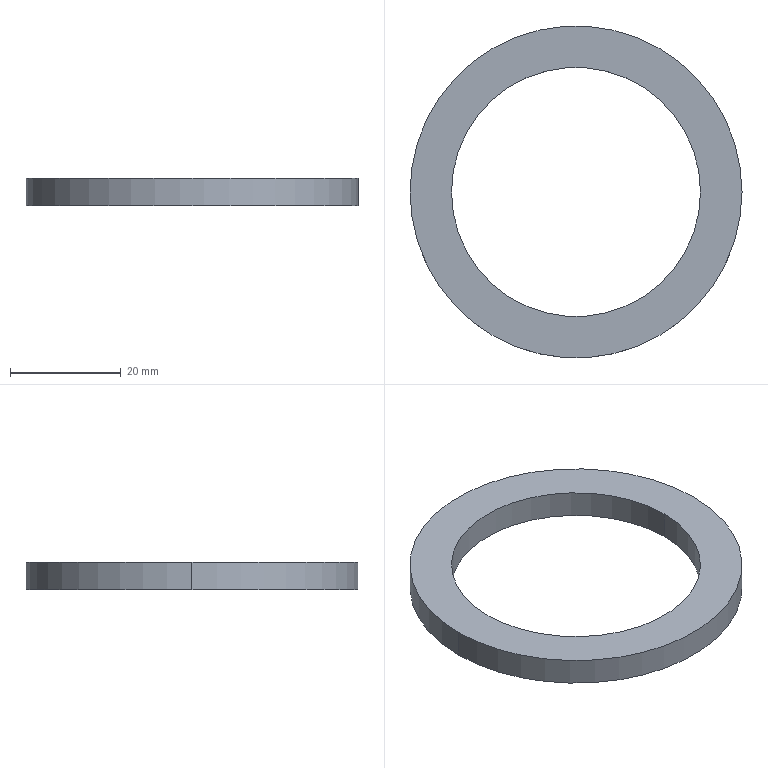Part | SolidWorks | features Extrusion 1 | 1 solid | 6 faces | box 60 x 60 x 5 mm | volume 6185 mm3 | cylinder 4 | plane 2 | commonest cylinder face diameters 45 x2 60 x2
STEP:
#1=CARTESIAN_POINT('',(-22.5,0.,5.));
#2=VERTEX_POINT('',#1);
#3=CARTESIAN_POINT('',(22.5,0.,5.));
#4=VERTEX_POINT('',#3);
#5=CARTESIAN_POINT('',(0.,0.,5.));
#6=DIRECTION('',(0.,0.,1.));
#7=DIRECTION('',(1.,0.,0.));
#8=AXIS2_PLACEMENT_3D('',#5,#6,#7);
#9=CIRCLE('',#8,22.5);
#10=EDGE_CURVE('',#2,#4,#9,.T.);
#11=ORIENTED_EDGE('',*,*,#10,.T.);
#12=CARTESIAN_POINT('',(22.5,0.,0.));
#13=VERTEX_POINT('',#12);
#14=CARTESIAN_POINT('',(22.5,0.,5.));
#15=DIRECTION('',(0.,0.,-1.));
#16=VECTOR('',#15,1000.);
#17=LINE('',#14,#16);
#18=EDGE_CURVE('',#4,#13,#17,.T.);
#19=ORIENTED_EDGE('',*,*,#18,.T.);
#20=CARTESIAN_POINT('',(-22.5,0.,0.));
#21=VERTEX_POINT('',#20);
#22=CARTESIAN_POINT('',(0.,0.,0.));
#23=DIRECTION('',(0.,0.,1.));
#24=DIRECTION('',(1.,0.,0.));
#25=AXIS2_PLACEMENT_3D('',#22,#23,#24);
#26=CIRCLE('',#25,22.5);
#27=EDGE_CURVE('',#21,#13,#26,.T.);
#28=ORIENTED_EDGE('',*,*,#27,.F.);
#29=CARTESIAN_POINT('',(-22.5,0.,5.));
#30=DIRECTION('',(0.,0.,-1.));
#31=VECTOR('',#30,1000.);
#32=LINE('',#29,#31);
#33=EDGE_CURVE('',#2,#21,#32,.T.);
#34=ORIENTED_EDGE('',*,*,#33,.F.);
#35=EDGE_LOOP('',(#11,#19,#28,#34));
#36=FACE_OUTER_BOUND('',#35,.T.);
#37=CARTESIAN_POINT('',(0.,0.,5.));
#38=DIRECTION('',(0.,0.,-1.));
#39=DIRECTION('',(-1.,0.,0.));
#40=AXIS2_PLACEMENT_3D('',#37,#38,#39);
#41=CYLINDRICAL_SURFACE('',#40,22.5);
#42=ADVANCED_FACE('',(#36),#41,.F.);
#43=CARTESIAN_POINT('',(30.,0.,5.));
#44=VERTEX_POINT('',#43);
#45=CARTESIAN_POINT('',(-30.,0.,5.));
#46=VERTEX_POINT('',#45);
#47=CARTESIAN_POINT('',(0.,0.,5.));
#48=DIRECTION('',(0.,0.,1.));
#49=DIRECTION('',(1.,0.,0.));
#50=AXIS2_PLACEMENT_3D('',#47,#48,#49);
#51=CIRCLE('',#50,30.);
#52=EDGE_CURVE('',#44,#46,#51,.T.);
#53=ORIENTED_EDGE('',*,*,#52,.F.);
#54=CARTESIAN_POINT('',(30.,0.,0.));
#55=VERTEX_POINT('',#54);
#56=CARTESIAN_POINT('',(30.,0.,5.));
#57=DIRECTION('',(0.,0.,-1.));
#58=VECTOR('',#57,1000.);
#59=LINE('',#56,#58);
#60=EDGE_CURVE('',#44,#55,#59,.T.);
#61=ORIENTED_EDGE('',*,*,#60,.T.);
#62=CARTESIAN_POINT('',(-30.,0.,0.));
#63=VERTEX_POINT('',#62);
#64=CARTESIAN_POINT('',(0.,0.,0.));
#65=DIRECTION('',(0.,0.,1.));
#66=DIRECTION('',(1.,0.,0.));
#67=AXIS2_PLACEMENT_3D('',#64,#65,#66);
#68=CIRCLE('',#67,30.);
#69=EDGE_CURVE('',#55,#63,#68,.T.);
#70=ORIENTED_EDGE('',*,*,#69,.T.);
#71=CARTESIAN_POINT('',(-30.,0.,5.));
#72=DIRECTION('',(0.,0.,-1.));
#73=VECTOR('',#72,1000.);
#74=LINE('',#71,#73);
#75=EDGE_CURVE('',#46,#63,#74,.T.);
#76=ORIENTED_EDGE('',*,*,#75,.F.);
#77=EDGE_LOOP('',(#53,#61,#70,#76));
#78=FACE_OUTER_BOUND('',#77,.T.);
#79=CARTESIAN_POINT('',(0.,0.,5.));
#80=DIRECTION('',(0.,0.,-1.));
#81=DIRECTION('',(-1.,0.,0.));
#82=AXIS2_PLACEMENT_3D('',#79,#80,#81);
#83=CYLINDRICAL_SURFACE('',#82,30.);
#84=ADVANCED_FACE('',(#78),#83,.T.);
#85=CARTESIAN_POINT('',(0.,0.,5.));
#86=DIRECTION('',(0.,0.,1.));
#87=DIRECTION('',(1.,0.,0.));
#88=AXIS2_PLACEMENT_3D('',#85,#86,#87);
#89=CIRCLE('',#88,30.);
#90=EDGE_CURVE('',#46,#44,#89,.T.);
#91=ORIENTED_EDGE('',*,*,#90,.T.);
#92=ORIENTED_EDGE('',*,*,#52,.T.);
#93=EDGE_LOOP('',(#91,#92));
#94=FACE_OUTER_BOUND('',#93,.T.);
#95=ORIENTED_EDGE('',*,*,#10,.F.);
#96=CARTESIAN_POINT('',(0.,0.,5.));
#97=DIRECTION('',(0.,0.,1.));
#98=DIRECTION('',(1.,0.,0.));
#99=AXIS2_PLACEMENT_3D('',#96,#97,#98);
#100=CIRCLE('',#99,22.5);
#101=EDGE_CURVE('',#4,#2,#100,.T.);
#102=ORIENTED_EDGE('',*,*,#101,.F.);
#103=EDGE_LOOP('',(#95,#102));
#104=FACE_BOUND('',#103,.T.);
#105=CARTESIAN_POINT('',(0.,0.,5.));
#106=DIRECTION('',(0.,0.,1.));
#107=DIRECTION('',(1.,0.,0.));
#108=AXIS2_PLACEMENT_3D('',#105,#106,#107);
#109=PLANE('',#108);
#110=ADVANCED_FACE('',(#94,#104),#109,.T.);
#111=CARTESIAN_POINT('',(0.,0.,0.));
#112=DIRECTION('',(0.,0.,1.));
#113=DIRECTION('',(1.,0.,0.));
#114=AXIS2_PLACEMENT_3D('',#111,#112,#113);
#115=CIRCLE('',#114,30.);
#116=EDGE_CURVE('',#63,#55,#115,.T.);
#117=ORIENTED_EDGE('',*,*,#116,.F.);
#118=ORIENTED_EDGE('',*,*,#69,.F.);
#119=EDGE_LOOP('',(#117,#118));
#120=FACE_OUTER_BOUND('',#119,.T.);
#121=ORIENTED_EDGE('',*,*,#27,.T.);
#122=CARTESIAN_POINT('',(0.,0.,0.));
#123=DIRECTION('',(0.,0.,1.));
#124=DIRECTION('',(1.,0.,0.));
#125=AXIS2_PLACEMENT_3D('',#122,#123,#124);
#126=CIRCLE('',#125,22.5);
#127=EDGE_CURVE('',#13,#21,#126,.T.);
#128=ORIENTED_EDGE('',*,*,#127,.T.);
#129=EDGE_LOOP('',(#121,#128));
#130=FACE_BOUND('',#129,.T.);
#131=CARTESIAN_POINT('',(0.,0.,0.));
#132=DIRECTION('',(0.,0.,1.));
#133=DIRECTION('',(1.,0.,0.));
#134=AXIS2_PLACEMENT_3D('',#131,#132,#133);
#135=PLANE('',#134);
#136=ADVANCED_FACE('',(#120,#130),#135,.F.);
#137=ORIENTED_EDGE('',*,*,#60,.F.);
#138=ORIENTED_EDGE('',*,*,#90,.F.);
#139=ORIENTED_EDGE('',*,*,#75,.T.);
#140=ORIENTED_EDGE('',*,*,#116,.T.);
#141=EDGE_LOOP('',(#137,#138,#139,#140));
#142=FACE_OUTER_BOUND('',#141,.T.);
#143=CARTESIAN_POINT('',(0.,0.,5.));
#144=DIRECTION('',(0.,0.,-1.));
#145=DIRECTION('',(-1.,0.,0.));
#146=AXIS2_PLACEMENT_3D('',#143,#144,#145);
#147=CYLINDRICAL_SURFACE('',#146,30.);
#148=ADVANCED_FACE('',(#142),#147,.T.);
#149=ORIENTED_EDGE('',*,*,#18,.F.);
#150=ORIENTED_EDGE('',*,*,#101,.T.);
#151=ORIENTED_EDGE('',*,*,#33,.T.);
#152=ORIENTED_EDGE('',*,*,#127,.F.);
#153=EDGE_LOOP('',(#149,#150,#151,#152));
#154=FACE_OUTER_BOUND('',#153,.T.);
#155=CARTESIAN_POINT('',(0.,0.,5.));
#156=DIRECTION('',(0.,0.,-1.));
#157=DIRECTION('',(-1.,0.,0.));
#158=AXIS2_PLACEMENT_3D('',#155,#156,#157);
#159=CYLINDRICAL_SURFACE('',#158,22.5);
#160=ADVANCED_FACE('',(#154),#159,.F.);
#161=CLOSED_SHELL('',(#42,#84,#110,#136,#148,#160));
#162=MANIFOLD_SOLID_BREP('',#161);
#163=CARTESIAN_POINT('',(0.,0.,0.));
#164=DIRECTION('',(0.,0.,1.));
#165=DIRECTION('',(1.,0.,0.));
#166=AXIS2_PLACEMENT_3D('',#163,#164,#165);
#167=(LENGTH_UNIT()NAMED_UNIT(*)SI_UNIT(.MILLI.,.METRE.));
#168=UNCERTAINTY_MEASURE_WITH_UNIT(LENGTH_MEASURE(0.00001),#167,'','');
#169=(NAMED_UNIT(*)PLANE_ANGLE_UNIT()SI_UNIT($,.RADIAN.));
#170=(NAMED_UNIT(*)SI_UNIT($,.STERADIAN.)SOLID_ANGLE_UNIT());
#171=(GEOMETRIC_REPRESENTATION_CONTEXT(3)GLOBAL_UNCERTAINTY_ASSIGNED_CONTEXT((#168))GLOBAL_UNIT_ASSIGNED_CONTEXT((#167,#169,#170))REPRESENTATION_CONTEXT('',''));
#172=ADVANCED_BREP_SHAPE_REPRESENTATION('',(#162,#166),#171);